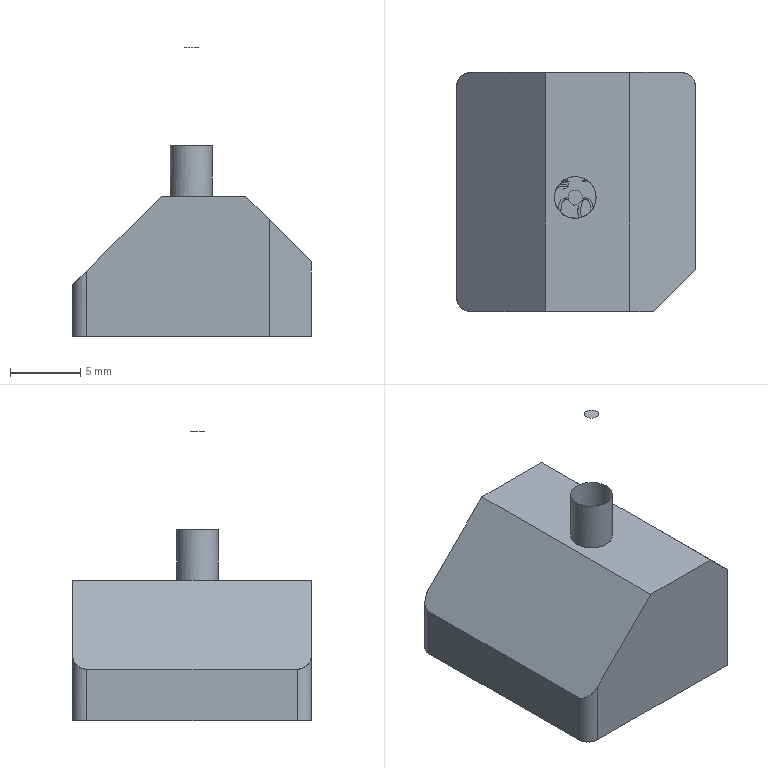NC program | PowerMill | posted with a generic post | part box 17 x 17 x 20.603 mm
Lines 61690 to 62415 of 69435:
N61787 M6
N61788 S18000 M03
N61789 G00 G90 X0.002 Y0.0
N61790 G43 Z9.803 H7
N61791
N61792 G05 P10000 R8
N61793 X9.5981 Y-6.0065
N61794 Z-14.5485
N61795 G01 Z-15.7485 F1200.0
N61796 X7.2501 Y-8.3545 Z-13.4005 F2000.0
N61797 X7.0261 Y-8.5078 Z-13.1711
N61798 X9.8459 Y-5.688 Z-15.9909
N61799 X9.9772 Y-5.486 Z-16.1229
N61800 X9.97 Y-5.4932 Z-16.1148
N61801 X9.9474 Y-5.5158 Z-16.0898
N61802 X9.9161 Y-5.5471 Z-16.058
N61803 X9.8562 Y-5.607 Z-15.9982
N61804 X9.775 Y-5.6881 Z-15.9171
N61805 X9.6405 Y-5.8227 Z-15.7827
N61806 X9.5138 Y-5.9494 Z-15.6555
N61807 X9.2093 Y-6.2539 Z-15.3515
N61808 X8.0778 Y-7.3854 Z-14.2199
N61809 X7.5441 Y-7.9191 Z-13.6862
N61810 X7.208 Y-8.2552 Z-13.3503
N61811 X7.0482 Y-8.415 Z-13.1914
N61812 X6.8884 Y-8.5748 Z-13.0327
N61813 X6.7529 Y-8.6395 Z-12.902
N61814 X6.8234 Y-8.5691 Z-12.9676
N61815 X6.8833 Y-8.5092 Z-13.0246
N61816 X6.9718 Y-8.4207 Z-13.113
N61817 X7.0894 Y-8.3031 Z-13.2309
N61818 X8.5064 Y-6.8861 Z-14.648
N61819 X9.2444 Y-6.1481 Z-15.3861
N61820 X9.5162 Y-5.8763 Z-15.6572
N61821 X9.6545 Y-5.738 Z-15.796
N61822 X9.7579 Y-5.6346 Z-15.8992
N61823 X9.8185 Y-5.574 Z-15.96
N61824 X9.875 Y-5.5175 Z-16.0163
N61825 X9.9261 Y-5.4663 Z-16.0688
N61826 X10.0013 Y-5.3912 Z-16.1496
N61827 X10.0032 Y-5.3893 Z-16.1516
N61828 X10.0226 Y-5.2992 Z-16.1743
N61829 X10.0195 Y-5.3023 Z-16.1706
N61830 X9.9961 Y-5.3256 Z-16.1426
N61831 X9.9739 Y-5.3478 Z-16.1183
N61832 X9.9271 Y-5.3947 Z-16.0692
N61833 X9.8819 Y-5.4399 Z-16.0231
N61834 X9.8289 Y-5.4929 Z-15.9705
N61835 X9.7574 Y-5.5644 Z-15.8987
N61836 X9.628 Y-5.6937 Z-15.7696
N61837 X9.2548 Y-6.067 Z-15.3965
N61838 X8.5168 Y-6.805 Z-14.6584
N61839 X7.0051 Y-8.3167 Z-13.1467
N61840 X6.892 Y-8.4297 Z-13.0332
N61841 X6.8083 Y-8.5135 Z-12.9497
N61842 X6.7465 Y-8.5752 Z-12.8912
N61843 X6.6718 Y-8.65 Z-12.822
N61844 X6.5956 Y-8.6554 Z-12.7464
N61845 X6.675 Y-8.5761 Z-12.8197
N61846 X6.7389 Y-8.5122 Z-12.8803
N61847 X6.8215 Y-8.4296 Z-12.9625
N61848 X6.9336 Y-8.3174 Z-13.0752
N61849 X9.5477 Y-5.7034 Z-15.6893
N61850 X9.8417 Y-5.4094 Z-15.9832
N61851 X9.9329 Y-5.3182 Z-16.0769
N61852 X10.0224 Y-5.2286 Z-16.1737
N61853 X10.0228 Y-5.2283 Z-16.1742
N61854 X10.0231 Y-5.1573 Z-16.174
N61855 X9.9404 Y-5.24 Z-16.0844
N61856 X9.8521 Y-5.3283 Z-15.9937
N61857 X6.7379 Y-8.4425 Z-12.8794
N61858 X6.6306 Y-8.5498 Z-12.7745
N61859 X6.5217 Y-8.6586 Z-12.6729
N61860 X6.451 Z-12.6022
N61861 X6.5593 Y-8.5503 Z-12.7032
N61862 X6.6658 Y-8.4439 Z-12.8073
N61863 X8.3044 Y-6.8052 Z-14.446
N61864 X9.067 Y-6.0426 Z-15.2087
N61865 X9.2959 Y-5.8138 Z-15.4371
N61866 X9.492 Y-5.6176 Z-15.6331
N61867 X9.6094 Y-5.5003 Z-15.7512
N61868 X9.7458 Y-5.3639 Z-15.887
N61869 X9.8058 Y-5.3038 Z-15.9474
N61870 X9.8617 Y-5.248 Z-16.0032
N61871 X9.9103 Y-5.1993 Z-16.0518
N61872 X9.9507 Y-5.1589 Z-16.0933
N61873 X9.9932 Y-5.1165 Z-16.1406
N61874 X10.0231 Y-5.0866 Z-16.1737
N61875 X10.0228 Y-5.0162 Z-16.174
N61876 X9.9785 Y-5.0604 Z-16.1235
N61877 X9.9395 Y-5.0995 Z-16.0815
N61878 X9.8992 Y-5.1398 Z-16.041
N61879 X9.8497 Y-5.1893 Z-15.991
N61880 X9.7933 Y-5.2457 Z-15.9348
N61881 X9.7215 Y-5.3174 Z-15.8627
N61882 X9.5857 Y-5.4532 Z-15.7276
N61883 X9.4743 Y-5.5647 Z-15.6151
N61884 X9.2716 Y-5.7673 Z-15.413
N61885 X9.0528 Y-5.9861 Z-15.1945
N61886 X8.3171 Y-6.7218 Z-14.4588
N61887 X6.5966 Y-8.4424 Z-12.7381
N61888 X6.4894 Y-8.5496 Z-12.6333
N61889 X6.3803 Y-8.6586 Z-12.5315
N61890 X6.3096 Z-12.4608
N61891 X6.4183 Y-8.55 Z-12.5621
N61892 X6.525 Y-8.4432 Z-12.6666
N61893 X8.2456 Y-6.7226 Z-14.3872
N61894 X9.0522 Y-5.916 Z-15.1938
N61895 X9.2696 Y-5.6986 Z-15.4111
N61896 X9.4749 Y-5.4933 Z-15.6157
N61897 X9.5834 Y-5.3848 Z-15.7253
N61898 X9.7066 Y-5.2616 Z-15.8479
N61899 X9.8038 Y-5.1645 Z-15.9453
N61900 X9.8576 Y-5.1106 Z-15.9989
N61901 X9.9067 Y-5.0615 Z-16.0487
N61902 X9.9542 Y-5.0141 Z-16.0968
N61903 X9.988 Y-4.9803 Z-16.134
N61904 X10.0226 Y-4.9456 Z-16.1742
N61905 X10.0225 Y-4.875 Z-16.1743
N61906 X9.9917 Y-4.9058 Z-16.1379
N61907 X9.9627 Y-4.9349 Z-16.106
N61908 X9.913 Y-4.9846 Z-16.055
N61909 X9.866 Y-5.0315 Z-16.0073
N61910 X9.8143 Y-5.0832 Z-15.9559
N61911 X9.7126 Y-5.1849 Z-15.8539
N61912 X9.5923 Y-5.3052 Z-15.7341
N61913 X9.4854 Y-5.4121 Z-15.6262
N61914 X9.2814 Y-5.6161 Z-15.4228
N61915 X9.065 Y-5.8325 Z-15.2067
N61916 X8.2562 Y-6.6413 Z-14.3978
N61917 X6.4536 Y-8.4439 Z-12.5951
N61918 X6.3472 Y-8.5503 Z-12.4911
N61919 X6.2389 Y-8.6586 Z-12.39
N61920 X6.1682 Z-12.3193
N61921 X6.2785 Y-8.5483 Z-12.4224
N61922 X6.387 Y-8.4398 Z-12.5286
N61923 X8.1895 Y-6.6373 Z-14.3311
N61924 X9.0288 Y-5.798 Z-15.1704
N61925 X9.2905 Y-5.5363 Z-15.4317
N61926 X9.5197 Y-5.3071 Z-15.6607
N61927 X9.631 Y-5.1958 Z-15.7728
N61928 X9.7694 Y-5.0574 Z-15.9104
N61929 X9.8296 Y-4.9972 Z-15.9712
N61930 X9.8785 Y-4.9483 Z-16.0198
N61931 X9.9228 Y-4.904 Z-16.0648
N61932 X9.9701 Y-4.8567 Z-16.1142
N61933 X9.9936 Y-4.8332 Z-16.1397
N61934 X10.0149 Y-4.8119 Z-16.1649
N61935 X10.0226 Y-4.8042 Z-16.1743
N61936 X10.0229 Y-4.7332 Z-16.1741
N61937 X9.9364 Y-4.8197 Z-16.0804
N61938 X9.8468 Y-4.9093 Z-15.9883
N61939 X9.5135 Y-5.2426 Z-15.6551
N61940 X6.4493 Y-8.3068 Z-12.5909
N61941 X6.3383 Y-8.4177 Z-12.4794
N61942 X6.2543 Y-8.5018 Z-12.3955
N61943 X6.1855 Y-8.5706 Z-12.3301
N61944 X6.0975 Y-8.6586 Z-12.2485
N61945 X6.0267 Z-12.1777
N61946 X6.1228 Y-8.5626 Z-12.2671
N61947 X6.1964 Y-8.489 Z-12.3375
N61948 X6.2842 Y-8.4012 Z-12.4254
N61949 X6.3955 Y-8.2899 Z-12.5371
N61950 X7.8378 Y-6.8476 Z-13.9793
N61951 X8.8324 Y-5.8529 Z-14.974
N61952 X9.0464 Y-5.6389 Z-15.1882
N61953 X9.3209 Y-5.3645 Z-15.4618
N61954 X9.5343 Y-5.1511 Z-15.6758
N61955 X9.6554 Y-5.0299 Z-15.7969
N61956 X9.7748 Y-4.9106 Z-15.9162
N61957 X9.8329 Y-4.8524 Z-15.9744
N61958 X9.8815 Y-4.8039 Z-16.0233
N61959 X9.932 Y-4.7534 Z-16.0737
N61960 X9.9696 Y-4.7157 Z-16.114
N61961 X10.0146 Y-4.6708 Z-16.1646
N61962 X10.023 Y-4.6624 Z-16.1738
N61963 X10.0226 Y-4.592 Z-16.1742
N61964 X9.9984 Y-4.6162 Z-16.1461
N61965 X9.9643 Y-4.6504 Z-16.1076
N61966 X9.9232 Y-4.6914 Z-16.0652
N61967 X9.874 Y-4.7407 Z-16.0153
N61968 X9.8244 Y-4.7902 Z-15.9661
N61969 X9.7711 Y-4.8436 Z-15.9122
N61970 X9.6477 Y-4.967 Z-15.7893
N61971 X9.5335 Y-5.0811 Z-15.6748
N61972 X9.324 Y-5.2907 Z-15.4649
N61973 X9.0641 Y-5.5505 Z-15.2059
N61974 X8.7554 Y-5.8592 Z-14.8969
N61975 X7.8502 Y-6.7644 Z-13.9918
N61976 X6.3442 Y-8.2704 Z-12.4858
N61977 X6.2307 Y-8.384 Z-12.372
N61978 X6.1379 Y-8.4768 Z-12.2789
N61979 X6.06 Y-8.5547 Z-12.204
N61980 X5.956 Y-8.6586 Z-12.1068
N61981 X5.8853 Y-8.6587 Z-12.0359
N61982 X6.0013 Y-8.5426 Z-12.1449
N61983 X6.0825 Y-8.4614 Z-12.2236
N61984 X6.1804 Y-8.3635 Z-12.322
N61985 X6.2856 Y-8.2583 Z-12.4271
N61986 X6.7127 Y-7.8313 Z-12.8542
N61987 X7.6646 Y-6.8793 Z-13.8062
N61988 X9.0729 Y-5.471 Z-15.2147
N61989 X9.3563 Y-5.1877 Z-15.4971
N61990 X9.565 Y-4.9789 Z-15.7066
N61991 X9.6789 Y-4.8651 Z-15.8203
N61992 X9.7925 Y-4.7514 Z-15.9338
N61993 X9.844 Y-4.7 Z-15.9856
N61994 X9.8915 Y-4.6524 Z-16.0331
N61995 X9.9388 Y-4.6052 Z-16.0812
N61996 X9.9751 Y-4.5689 Z-16.1192
N61997 X10.005 Y-4.5389 Z-16.1537
N61998 X10.0226 Y-4.5214 Z-16.1743
N61999 X10.0227 Y-4.4505 Z-16.1742
N62000 X10.0096 Y-4.4637 Z-16.1596
N62001 X9.9448 Y-4.5284 Z-16.088
N62002 X9.8987 Y-4.5745 Z-16.0398
N62003 X9.8382 Y-4.635 Z-15.9798
N62004 X6.0491 Y-8.4242 Z-12.1907
N62005 X5.95 Y-8.5232 Z-12.0919
N62006 X5.8773 Y-8.596 Z-12.0219
N62007 X5.8146 Y-8.6587 Z-11.9653
N62008 X5.7439 Z-11.8949
N62009 X5.8124 Y-8.5902 Z-11.9576
N62010 X5.8564 Y-8.5461 Z-11.9988
N62011 X5.89 Y-8.5125 Z-12.0318
N62012 X5.9235 Y-8.479 Z-12.0651
N62013 X5.9569 Y-8.4456 Z-12.0985
N62014 X5.9904 Y-8.4122 Z-12.1319
N62015 X6.0238 Y-8.3788 Z-12.1653
N62016 X8.6308 Y-5.7717 Z-14.7724
N62017 X9.266 Y-5.1365 Z-15.4076
N62018 X9.5463 Y-4.8563 Z-15.6879
N62019 X9.7507 Y-4.6518 Z-15.8923
N62020 X9.8723 Y-4.5303 Z-16.0138
N62021 X9.9504 Y-4.4522 Z-16.0945
N62022 X10.0228 Y-4.3797 Z-16.1739
N62023 X10.0226 Y-4.3093 Z-16.1743
N62024 X10.0201 Y-4.3117 Z-16.1715
N62025 X9.9647 Y-4.3672 Z-16.1088
N62026 X9.9062 Y-4.4256 Z-16.0478
N62027 X9.7422 Y-4.5896 Z-15.8838
N62028 X9.4962 Y-4.8357 Z-15.6378
N62029 X8.9425 Y-5.3893 Z-15.0841
N62030 X5.8897 Y-8.4421 Z-12.0312
N62031 X5.7822 Y-8.5496 Z-11.9261
N62032 X5.6731 Y-8.6587 Z-11.8242
N62033 X5.6024 Z-11.7532
N62034 X5.7047 Y-8.5564 Z-11.8488
N62035 X5.782 Y-8.4791 Z-11.9231
N62036 X5.8727 Y-8.3884 Z-12.0141
N62037 X5.9778 Y-8.2834 Z-12.1192
N62038 X6.3937 Y-7.8674 Z-12.5353
N62039 X9.8597 Y-4.4014 Z-16.0012
N62040 X9.9461 Y-4.315 Z-16.0901
N62041 X10.0233 Y-4.2378 Z-16.1738
N62042 X10.0226 Y-4.1678 Z-16.1743
N62043 X10.0201 Y-4.1703 Z-16.1714
N62044 X9.9579 Y-4.2325 Z-16.102
N62045 X9.8927 Y-4.2977 Z-16.0343
N62046 X9.7287 Y-4.4617 Z-15.8703
N62047 X9.4006 Y-4.7898 Z-15.5423
N62048 X8.7446 Y-5.4458 Z-14.8862
N62049 X5.7797 Y-8.4107 Z-11.9213
N62050 X5.6736 Y-8.5168 Z-11.8153
N62051 X5.6013 Y-8.5891 Z-11.7455
N62052 X5.5402 Y-8.6502 Z-11.69
N62053 X5.4781 Y-8.6416 Z-11.6273
N62054 X5.5198 Y-8.5999 Z-11.6647
N62055 X5.5608 Y-8.5589 Z-11.7036
N62056 X5.6015 Y-8.5182 Z-11.7431
N62057 X5.6856 Y-8.4341 Z-11.8267
N62058 X5.8032 Y-8.3165 Z-11.9448
N62059 X7.8382 Y-6.2815 Z-13.9798
N62060 X9.8578 Y-4.2619 Z-15.9994
N62061 X9.9447 Y-4.175 Z-16.0887
N62062 X10.0232 Y-4.0964 Z-16.1739
N62063 X10.0226 Y-4.0264 Z-16.1742
N62064 X10.0203 Y-4.0287 Z-16.1716
N62065 X9.957 Y-4.092 Z-16.1011
N62066 X9.8906 Y-4.1584 Z-16.0322
N62067 X9.7266 Y-4.3224 Z-15.8682
N62068 X9.3986 Y-4.6504 Z-15.5402
N62069 X8.8246 Y-5.2244 Z-14.9661
N62070 X6.8458 Y-7.2032 Z-12.9874
N62071 X6.4185 Y-7.6305 Z-12.5601
N62072 X6.0439 Y-8.0051 Z-12.1851
N62073 X5.87 Y-8.1789 Z-12.0117
N62074 X5.689 Y-8.36 Z-11.8301
N62075 X5.5984 Y-8.4506 Z-11.7405
N62076 X5.5076 Y-8.5414 Z-11.6516
N62077 X5.4159 Y-8.6331 Z-11.5643
N62078 X5.382 Y-8.5963 Z-11.5274
N62079 X5.4532 Y-8.5251 Z-11.5969
N62080 X5.5243 Y-8.454 Z-11.6668
N62081 X5.5952 Y-8.3831 Z-11.7369
N62082 X5.666 Y-8.3123 Z-11.8073
N62083 X5.9062 Y-8.0721 Z-12.0479
N62084 X6.1282 Y-7.8501 Z-12.2695
N62085 X6.6142 Y-7.3641 Z-12.7558
N62086 X8.3809 Y-5.5974 Z-14.5224
N62087 X9.8647 Y-4.1135 Z-16.0063
N62088 X9.9475 Y-4.0308 Z-16.0915
N62089 X10.023 Y-3.9552 Z-16.1737
N62090 X10.0226 Y-3.885 Z-16.1743
N62091 X10.0208 Y-3.8868 Z-16.1721
N62092 X9.9677 Y-3.9399 Z-16.1117
N62093 X9.912 Y-3.9955 Z-16.0536
N62094 X9.748 Y-4.1596 Z-15.8896
N62095 X9.42 Y-4.4876 Z-15.5616
N62096 X8.846 Y-5.0616 Z-14.9875
N62097 X6.4678 Y-7.4398 Z-12.6094
N62098 X5.9091 Y-7.9984 Z-12.0508
N62099 X5.8469 Y-8.0606 Z-11.9887
N62100 X5.7848 Y-8.1227 Z-11.9265
N62101 X5.7227 Y-8.1849 Z-11.8642
N62102 X5.6606 Y-8.247 Z-11.802
N62103 X5.5984 Y-8.3091 Z-11.7398
N62104 X5.5363 Y-8.3713 Z-11.6776
N62105 X5.4741 Y-8.4335 Z-11.6156
N62106 X5.4117 Y-8.4958 Z-11.5538
N62107 X5.3491 Y-8.5584 Z-11.4925
N62108 X5.3211 Y-8.5157 Z-11.4632
N62109 X5.9951 Y-7.8417 Z-12.1367
N62110 X6.6689 Y-7.1679 Z-12.8105
N62111 X8.8099 Y-5.027 Z-14.9515
N62112 X9.3839 Y-4.453 Z-15.5255
N62113 X9.7119 Y-4.1249 Z-15.8535
N62114 X9.876 Y-3.9609 Z-16.0175
N62115 X9.9513 Y-3.8856 Z-16.0954
N62116 X10.0228 Y-3.8141 Z-16.174
N62117 X10.023 Y-3.7432 Z-16.1741
N62118 X9.9377 Y-3.8285 Z-16.0817
N62119 X9.8485 Y-3.9177 Z-15.99
N62120 X5.2969 Y-8.4692 Z-11.4385
N62121 X5.2726 Y-8.4229 Z-11.4143
N62122 X5.8386 Y-7.8569 Z-11.9801
N62123 X8.0944 Y-5.601 Z-14.236
N62124 X9.0385 Y-4.657 Z-15.1802
N62125 X9.2994 Y-4.3961 Z-15.4404
N62126 X9.5199 Y-4.1756 Z-15.6609
N62127 X9.6315 Y-4.0639 Z-15.7733
N62128 X9.7651 Y-3.9304 Z-15.9061
N62129 X9.8165 Y-3.8789 Z-15.9581
N62130 X9.8674 Y-3.8281 Z-16.0087
N62131 X9.9137 Y-3.7818 Z-16.0557
N62132 X9.9642 Y-3.7312 Z-16.1077
N62133 X9.9922 Y-3.7032 Z-16.1384
N62134 X10.0225 Y-3.6729 Z-16.1743
N62135 X10.0231 Y-3.6016 Z-16.1737
N62136 X9.9477 Y-3.6771 Z-16.0918
N62137 X9.8623 Y-3.7624 Z-16.0039
N62138 X9.6983 Y-3.9264 Z-15.8399
N62139 X9.3702 Y-4.2545 Z-15.5119
N62140 X8.7962 Y-4.8285 Z-14.9378
N62141 X6.6847 Y-6.9401 Z-12.8262
N62142 X5.784 Y-7.8407 Z-11.9257
N62143 X5.5162 Y-8.1085 Z-11.6577
N62144 X5.2481 Y-8.3766 Z-11.3903
N62145 X5.2235 Y-8.3305 Z-11.3664
N62146 X5.3564 Y-8.1976 Z-11.4978
N62147 X5.4888 Y-8.0652 Z-11.6302
N62148 X5.6211 Y-7.9329 Z-11.7629
N62149 X5.7535 Y-7.8005 Z-11.8953
N62150 X6.4131 Y-7.1409 Z-12.5547
N62151 X8.8434 Y-4.7106 Z-14.985
N62152 X9.4174 Y-4.1366 Z-15.5591
N62153 X9.7455 Y-3.8085 Z-15.8871
N62154 X9.9095 Y-3.6445 Z-16.0511
N62155 X9.9663 Y-3.5877 Z-16.1103
N62156 X10.0205 Y-3.5335 Z-16.1719
N62157 X10.0226 Y-3.5314 Z-16.1743
N62158 Y-3.4607
N62159 X10.0203 Y-3.463 Z-16.1716
N62160 X9.9651 Y-3.5182 Z-16.1092
N62161 X9.9073 Y-3.576 Z-16.0489
N62162 X9.7433 Y-3.74 Z-15.8849
N62163 X9.4153 Y-4.068 Z-15.5569
N62164 X8.8413 Y-4.642 Z-14.9828
N62165 X6.3811 Y-7.1022 Z-12.5227
N62166 X5.8861 Y-7.5972 Z-12.0274
N62167 X5.6196 Y-7.8637 Z-11.7612
N62168 X5.3691 Y-8.1142 Z-11.5109
N62169 X5.2006 Y-8.2827 Z-11.3445
N62170 X5.1776 Y-8.235 Z-11.3232
N62171 X5.2516 Y-8.161 Z-11.3939
N62172 X5.3221 Y-8.0905 Z-11.4635
N62173 X5.4002 Y-8.0124 Z-11.5416
N62174 X5.609 Y-7.8036 Z-11.7506
N62175 X5.8207 Y-7.5919 Z-11.9619
N62176 X6.2956 Y-7.117 Z-12.4373
N62177 X6.8187 Y-6.5938 Z-12.9603
N62178 X8.8135 Y-4.5991 Z-14.955
N62179 X9.3875 Y-4.0251 Z-15.5291
N62180 X9.7155 Y-3.6971 Z-15.8571
N62181 X9.8795 Y-3.5331 Z-16.0211
N62182 X9.9525 Y-3.4601 Z-16.0966
N62183 X10.0221 Y-3.3905 Z-16.1734
N62184 X10.0227 Y-3.3899 Z-16.1741
N62185 X10.023 Y-3.3189
N62186 X9.9381 Y-3.4038 Z-16.0821
N62187 X9.8489 Y-3.493 Z-15.9905
N62188 X7.1169 Y-6.2249 Z-13.2585
N62189 X5.867 Y-7.4749 Z-12.0085
N62190 X5.6084 Y-7.7335 Z-11.75
N62191 X5.3873 Y-7.9546 Z-11.5286
N62192 X5.3202 Y-8.0216 Z-11.4617
N62193 X5.2638 Y-8.078 Z-11.4056
N62194 X5.2023 Y-8.1396 Z-11.3453
N62195 X5.1787 Y-8.1632 Z-11.3232
N62196 X5.1544 Y-8.1875 Z-11.3024
N62197 X5.1396 Y-8.1316 Z-11.2892
N62198 X5.2416 Y-8.0295 Z-11.3853
N62199 X5.351 Y-7.9202 Z-11.4926
N62200 X5.6356 Y-7.6356 Z-11.7772
N62201 X7.1496 Y-6.1216 Z-13.2912
N62202 X8.7518 Y-4.5194 Z-14.8933
N62203 X9.4078 Y-3.8634 Z-15.5494
N62204 X9.7358 Y-3.5353 Z-15.8774
N62205 X9.8998 Y-3.3713 Z-16.0414
N62206 X9.9612 Y-3.31 Z-16.1053
N62207 X10.02 Y-3.2511 Z-16.1714
N62208 X10.0225 Y-3.2486 Z-16.1743
N62209 X10.0226 Y-3.1779
N62210 X10.0201 Y-3.1804 Z-16.1714
N62211 X9.9629 Y-3.2375 Z-16.107
N62212 X9.9032 Y-3.2973 Z-16.0448
N62213 X9.7392 Y-3.4613 Z-15.8808
N62214 X9.4111 Y-3.7893 Z-15.5528
N62215 X8.8371 Y-4.3633 Z-14.9787
N62216 X5.3264 Y-7.8741 Z-11.468
N62217 X5.2313 Y-7.9691 Z-11.3746
N62218 X5.1347 Y-8.0657 Z-11.2845
N62219 X5.1297 Y-8.0001 Z-11.2802
N62220 X5.1712 Y-7.9585 Z-11.3174
N62221 X5.2109 Y-7.9188 Z-11.3532
N62222 X5.2543 Y-7.8755 Z-11.396
N62223 X5.3045 Y-7.8253 Z-11.4458
N62224 X5.3722 Y-7.7575 Z-11.5138
N62225 X5.4428 Y-7.6869 Z-11.5841
N62226 X5.6969 Y-7.4329 Z-11.8385
N62227 X6.7815 Y-6.3482 Z-12.9231
N62228 X8.3541 Y-4.7756 Z-14.4957
N62229 X9.1694 Y-3.9603 Z-15.3109
N62230 X9.3543 Y-3.7754 Z-15.4958
N62231 X9.5404 Y-3.5894 Z-15.681
N62232 X9.6332 Y-3.4966 Z-15.7747
N62233 X9.7157 Y-3.4141 Z-15.8573
N62234 X9.7972 Y-3.3326 Z-15.9388
N62235 X9.8518 Y-3.278 Z-15.9931
N62236 X9.9021 Y-3.2276 Z-16.044
N62237 X9.9487 Y-3.181 Z-16.0911
N62238 X9.9857 Y-3.1441 Z-16.1315
N62239 X10.0227 Y-3.107 Z-16.1741
N62240 X10.023 Y-3.0361
N62241 X9.9378 Y-3.1212 Z-16.0818
N62242 X9.8486 Y-3.2105 Z-15.9901
N62243 X8.5365 Y-4.5226 Z-14.678
N62244 X6.3019 Y-6.7571 Z-12.4435
N62245 X5.7416 Y-7.3175 Z-11.8832
N62246 X5.339 Y-7.72 Z-11.4806
N62247 X5.2687 Y-7.7904 Z-11.4103
N62248 X5.1983 Y-7.8607 Z-11.3425
N62249 X5.1272 Y-7.9319 Z-11.2787
N62250 X5.1271 Y-7.8612
N62251 X5.1552 Y-7.8331 Z-11.3022
N62252 X5.1827 Y-7.8057 Z-11.327
N62253 X5.2399 Y-7.7484 Z-11.3818
N62254 X5.2886 Y-7.6997 Z-11.4298
N62255 X5.3525 Y-7.6358 Z-11.494
N62256 X5.6373 Y-7.351 Z-11.7789
N62257 X7.3084 Y-5.6799 Z-13.45
N62258 X8.7535 Y-4.2348 Z-14.8951
N62259 X9.4096 Y-3.5788 Z-15.5512
N62260 X9.7376 Y-3.2507 Z-15.8792
N62261 X9.9016 Y-3.0867 Z-16.0432
N62262 X9.9621 Y-3.0262 Z-16.1062
N62263 X10.0201 Y-2.9682 Z-16.1714
N62264 X10.0226 Y-2.9658 Z-16.1743
N62265 Y-2.895
N62266 X10.0202 Y-2.8974 Z-16.1715
N62267 X9.9645 Y-2.9531 Z-16.1086
N62268 X9.9062 Y-3.0114 Z-16.0478
N62269 X9.7422 Y-3.1754 Z-15.8838
N62270 X9.4141 Y-3.5035 Z-15.5558
N62271 X8.8401 Y-4.0775 Z-14.9817
N62272 X5.3147 Y-7.6029 Z-11.4563
N62273 X5.2217 Y-7.6959 Z-11.3657
N62274 X5.1272 Y-7.7904 Z-11.2785
N62275 X5.1275 Y-7.7194 Z-11.2781
N62276 X5.2173 Y-7.6296 Z-11.361
N62277 X5.3056 Y-7.5413 Z-11.4472
N62278 X8.8236 Y-4.0233 Z-14.9652
N62279 X9.3976 Y-3.4493 Z-15.5392
N62280 X9.7256 Y-3.1213 Z-15.8672
N62281 X9.8896 Y-2.9573 Z-16.0312
N62282 X9.9566 Y-2.8903 Z-16.1007
N62283 X10.0203 Y-2.8266 Z-16.1716
N62284 X10.0226 Y-2.8243 Z-16.1742
N62285 X10.0228 Y-2.7534 Z-16.174
N62286 X9.951 Y-2.8252 Z-16.0951
N62287 X9.8753 Y-2.9009 Z-16.0168
N62288 X9.7112 Y-3.065 Z-15.8528
N62289 X9.3832 Y-3.393 Z-15.5248
N62290 X8.8092 Y-3.967 Z-14.9508
N62291 X6.9764 Y-5.7997 Z-13.118
N62292 X5.693 Y-7.0832 Z-11.8346
N62293 X5.4365 Y-7.3397 Z-11.5778
N62294 X5.3666 Y-7.4096 Z-11.5082
N62295 X5.3008 Y-7.4754 Z-11.4422
N62296 X5.2505 Y-7.5257 Z-11.3922
N62297 X5.2076 Y-7.5686 Z-11.35
N62298 X5.1684 Y-7.6078 Z-11.3148
N62299 X5.1274 Y-7.6488 Z-11.2783
N62300 X5.1273 Y-7.5782 Z-11.2785
N62301 X5.1794 Y-7.5261 Z-11.324
N62302 X5.2194 Y-7.4861 Z-11.3616
N62303 X5.2781 Y-7.4274 Z-11.4197
N62304 X5.3328 Y-7.3727 Z-11.4743
N62305 X5.4011 Y-7.3044 Z-11.5425
N62306 X5.6545 Y-7.051 Z-11.7961
N62307 X5.9552 Y-6.7503 Z-12.0968
N62308 X7.5705 Y-5.135 Z-13.7121
N62309 X8.8006 Y-3.9049 Z-14.9422
N62310 X9.3746 Y-3.3309 Z-15.5162
N62311 X9.7026 Y-3.0028 Z-15.8442
N62312 X9.8666 Y-2.8388 Z-16.0082
N62313 X9.9486 Y-2.7569 Z-16.0927
N62314 X10.023 Y-2.6825 Z-16.1738
N62315 X10.0232 Y-2.6116 Z-16.1736
N62316 X9.9474 Y-2.6874 Z-16.0915
N62317 X9.8608 Y-2.774 Z-16.0024
N62318 X9.6968 Y-2.938 Z-15.8384
N62319 X9.3687 Y-3.266 Z-15.5104
N62320 X8.7947 Y-3.84 Z-14.9363
N62321 X7.5647 Y-5.0701 Z-13.7062
N62322 X5.9511 Y-6.6837 Z-12.0926
N62323 X5.648 Y-6.9868 Z-11.7896
N62324 X5.3946 Y-7.2402 Z-11.536
N62325 X5.3272 Y-7.3075 Z-11.4686
N62326 X5.2747 Y-7.3601 Z-11.4163
N62327 X5.2189 Y-7.4159 Z-11.361
N62328 X5.1786 Y-7.4562 Z-11.3233
N62329 X5.1272 Y-7.5075 Z-11.2785
N62330 Y-7.4369 Z-11.2786
N62331 X5.1757 Y-7.3883 Z-11.3207
N62332 X5.2141 Y-7.3499 Z-11.3565
N62333 X5.2711 Y-7.2929 Z-11.4128
N62334 X5.3244 Y-7.2397 Z-11.4658
N62335 X5.3908 Y-7.1732 Z-11.5322
N62336 X5.6429 Y-6.9211 Z-11.7845
N62337 X5.9384 Y-6.6257 Z-12.0799
N62338 X7.3445 Y-5.2196 Z-13.486
N62339 X9.8549 Y-2.7092 Z-15.9965
N62340 X9.9424 Y-2.6216 Z-16.0865
N62341 X10.0232 Y-2.5409 Z-16.1739
N62342 X10.023 Y-2.4703 Z-16.174
N62343 X9.9387 Y-2.5547 Z-16.0827
N62344 X9.8498 Y-2.6436 Z-15.9914
N62345 X7.3849 Y-5.1084 Z-13.5265
N62346 X5.9383 Y-6.555 Z-12.0799
N62347 X5.6392 Y-6.8541 Z-11.7809
N62348 X5.3854 Y-7.1079 Z-11.5268
N62349 X5.3196 Y-7.1737 Z-11.461
N62350 X5.2671 Y-7.2262 Z-11.4088
N62351 X5.2101 Y-7.2833 Z-11.3527
N62352 X5.1733 Y-7.3201 Z-11.3184
N62353 X5.1271 Y-7.3662 Z-11.2786
N62354 Y-7.2955
N62355 X5.1727 Y-7.2499 Z-11.3179
N62356 X5.2091 Y-7.2135 Z-11.3517
N62357 X5.2662 Y-7.1565 Z-11.4078
N62358 X5.3184 Y-7.1042 Z-11.4598
N62359 X5.3841 Y-7.0385 Z-11.5255
N62360 X5.6386 Y-6.784 Z-11.7802
N62361 X5.9391 Y-6.4835 Z-12.0807
N62362 X7.4167 Y-5.0059 Z-13.5583
N62363 X9.8485 Y-2.5741 Z-15.9901
N62364 X9.9378 Y-2.4848 Z-16.0819
N62365 X10.023 Y-2.3997 Z-16.1741
N62366 Y-2.329
N62367 X9.9374 Y-2.4145 Z-16.0814
N62368 X9.8479 Y-2.504 Z-15.9895
N62369 X7.4097 Y-4.9423 Z-13.5512
N62370 X5.939 Y-6.4129 Z-12.0806
N62371 X5.6383 Y-6.7136 Z-11.7799
N62372 X5.3835 Y-6.9684 Z-11.5249
N62373 X5.3179 Y-7.034 Z-11.4593
N62374 X5.2657 Y-7.0862 Z-11.4074
N62375 X5.2086 Y-7.1433 Z-11.3513
N62376 X5.1724 Y-7.1795 Z-11.3177
N62377 X5.1271 Y-7.2248 Z-11.2786
N62378 Y-7.1541
N62379 X5.1745 Y-7.1067 Z-11.3206
N62380 X5.2211 Y-7.0602 Z-11.3643
N62381 X5.2672 Y-7.014 Z-11.4089
N62382 X5.313 Y-6.9683 Z-11.4543
N62383 X5.3785 Y-6.9027 Z-11.5199
N62384 X5.6302 Y-6.651 Z-11.7718
N62385 X5.9314 Y-6.3498 Z-12.073
N62386 X7.4058 Y-4.8754 Z-13.5474
N62387 X9.8474 Y-2.4339 Z-15.989
N62388 X9.937 Y-2.3442 Z-16.0811
N62389 X10.0229 Y-2.2583 Z-16.1741
N62390 Y-2.1876
N62391 X9.937 Y-2.2735 Z-16.0811
N62392 X9.8474 Y-2.3631 Z-15.989
N62393 X7.4256 Y-4.7849 Z-13.5672
N62394 X5.9398 Y-6.2707 Z-12.0814
N62395 X5.6383 Y-6.5722 Z-11.7799
N62396 X5.383 Y-6.8275 Z-11.5244
N62397 X5.3174 Y-6.8931 Z-11.4588
N62398 X5.2653 Y-6.9452 Z-11.407
N62399 X5.2082 Y-7.0023 Z-11.3509
N62400 X5.1722 Y-7.0383 Z-11.3174
N62401 X5.1271 Y-7.0834 Z-11.2786
N62402 Y-7.0127
N62403 X5.1722 Y-6.9676 Z-11.3174
N62404 X5.2082 Y-6.9316 Z-11.3509
N62405 X5.2652 Y-6.8745 Z-11.4069
N62406 X5.3174 Y-6.8224 Z-11.4587
N62407 X5.3829 Y-6.7569 Z-11.5243
N62408 X5.6384 Y-6.5014 Z-11.78
N62409 X5.9403 Y-6.1995 Z-12.0819
N62410 X7.4224 Y-4.7174 Z-13.564
N62411 X9.8474 Y-2.2924 Z-15.989
N62412 X9.937 Y-2.2028 Z-16.0811
N62413 X10.0229 Y-2.1169 Z-16.1741
N62414 Y-2.0461
N62415 X9.937 Y-2.1321 Z-16.0811
N62416 X9.8474 Y-2.2217 Z-15.989
N62417 X7.4166 Y-4.6525 Z-13.5582
N62418 X5.9301 Y-6.1389 Z-12.0717
N62419 X5.6287 Y-6.4404 Z-11.7703
N62420 X5.3776 Y-6.6915 Z-11.519
N62421 X5.312 Y-6.7571 Z-11.4533
N62422 X5.2598 Y-6.8093 Z-11.4017
N62423 X5.1859 Y-6.8832 Z-11.3314
N62424 X5.1271 Y-6.942 Z-11.2786
N62425 Y-6.8713
N62426 X5.1978 Y-6.8006 Z-11.342
N62427 X5.2677 Y-6.7307 Z-11.4093
N62428 X5.3377 Y-6.6607 Z-11.4792
N62429 X5.7273 Y-6.2711 Z-11.8689
N62430 X6.2625 Y-5.7359 Z-12.404
N62431 X8.0924 Y-3.906 Z-14.2339
N62432 X9.8474 Y-2.151 Z-15.989
N62433 X9.9371 Y-2.0613 Z-16.0812
N62434 X10.0229 Y-1.9754 Z-16.1741
N62435 Y-1.9047
N62436 X9.937 Y-1.9907 Z-16.0811
N62437 X9.8474 Y-2.0803 Z-15.989
N62438 X7.409 Y-4.5187 Z-13.5505
N62439 X5.9392 Y-5.9885 Z-12.0807
N62440 X5.638 Y-6.2897 Z-11.7796
N62441 X5.3829 Y-6.5447 Z-11.5243
N62442 X5.3174 Y-6.6103 Z-11.4588
N62443 X5.2653 Y-6.6624 Z-11.407
N62444 X5.2082 Y-6.7195 Z-11.3509
N62445 X5.1722 Y-6.7555 Z-11.3174
N62446 X5.1271 Y-6.8006 Z-11.2786
N62447 Y-6.7298
N62448 X5.1976 Y-6.6593 Z-11.3418
N62449 X5.2675 Y-6.5894 Z-11.4091
N62450 X5.3378 Y-6.5192 Z-11.4793
N62451 X5.6547 Y-6.2023 Z-11.7963
N62452 X6.2363 Y-5.6206 Z-12.3779
N62453 X7.7152 Y-4.1417 Z-13.8568
N62454 X9.8474 Y-2.0096 Z-15.9889
N62455 X9.937 Y-1.92 Z-16.081
N62456 X10.0229 Y-1.834 Z-16.1741
N62457 Y-1.7633
N62458 X9.937 Y-1.8492 Z-16.081
N62459 X9.8474 Y-1.9389 Z-15.989
N62460 X7.3975 Y-4.3887 Z-13.5391
N62461 X5.9093 Y-5.8769 Z-12.0509
N62462 X5.6077 Y-6.1785 Z-11.7493
N62463 X5.3652 Y-6.4211 Z-11.5067
N62464 X5.2997 Y-6.4865 Z-11.4409
N62465 X5.2571 Y-6.5291 Z-11.3991
N62466 X5.2141 Y-6.5721 Z-11.3582
N62467 X5.1709 Y-6.6154 Z-11.3179
N62468 X5.1271 Y-6.6591 Z-11.2786
N62469 Y-6.5884
N62470 X5.1722 Y-6.5434 Z-11.3174
N62471 X5.2082 Y-6.5073 Z-11.3509
N62472 X5.2652 Y-6.4503 Z-11.4069
N62473 X5.3174 Y-6.3982 Z-11.4587
N62474 X5.3829 Y-6.3326 Z-11.5244
N62475 X5.6383 Y-6.0772 Z-11.78
N62476 X5.9401 Y-5.7754 Z-12.0817
N62477 X7.4208 Y-4.2948 Z-13.5624
N62478 X9.8474 Y-1.8682 Z-15.989
N62479 X9.937 Y-1.7785 Z-16.0811
N62480 X10.0229 Y-1.6926 Z-16.1741
N62481 Y-1.6219
N62482 X9.937 Y-1.7078 Z-16.0811
N62483 X9.8474 Y-1.7975 Z-15.989
N62484 X7.423 Y-4.2218 Z-13.5646
N62485 X5.9398 Y-5.7051 Z-12.0813
N62486 X5.6382 Y-6.0066 Z-11.7799
N62487 X5.383 Y-6.2619 Z-11.5244
N62488 X5.3174 Y-6.3274 Z-11.4587
N62489 X5.2653 Y-6.3796 Z-11.4069
N62490 X5.2082 Y-6.4366 Z-11.3509
N62491 X5.1722 Y-6.4727 Z-11.3174
N62492 X5.1271 Y-6.5177 Z-11.2786
N62493 Y-6.447
N62494 X5.1722 Y-6.4019 Z-11.3174
N62495 X5.2082 Y-6.3659 Z-11.3509
N62496 X5.2653 Y-6.3088 Z-11.407
N62497 X5.3167 Y-6.2574 Z-11.4581
N62498 X5.3788 Y-6.1953 Z-11.5202
N62499 X5.5575 Y-6.0166 Z-11.6992
N62500 X5.7477 Y-5.8264 Z-11.8892
N62501 X6.2434 Y-5.3307 Z-12.3851
N62502 X7.3951 Y-4.179 Z-13.5367
N62503 X9.8474 Y-1.7267 Z-15.989
N62504 X9.9369 Y-1.6372 Z-16.0809
N62505 X10.0229 Y-1.5512 Z-16.1741
N62506 Y-1.4805
N62507 X9.937 Y-1.5664 Z-16.0811
N62508 X9.8474 Y-1.656 Z-15.989
N62509 X7.4108 Y-4.0926 Z-13.5524
N62510 X5.9392 Y-5.5642 Z-12.0808
N62511 X5.638 Y-5.8654 Z-11.7796
N62512 X5.3829 Y-6.1205 Z-11.5243